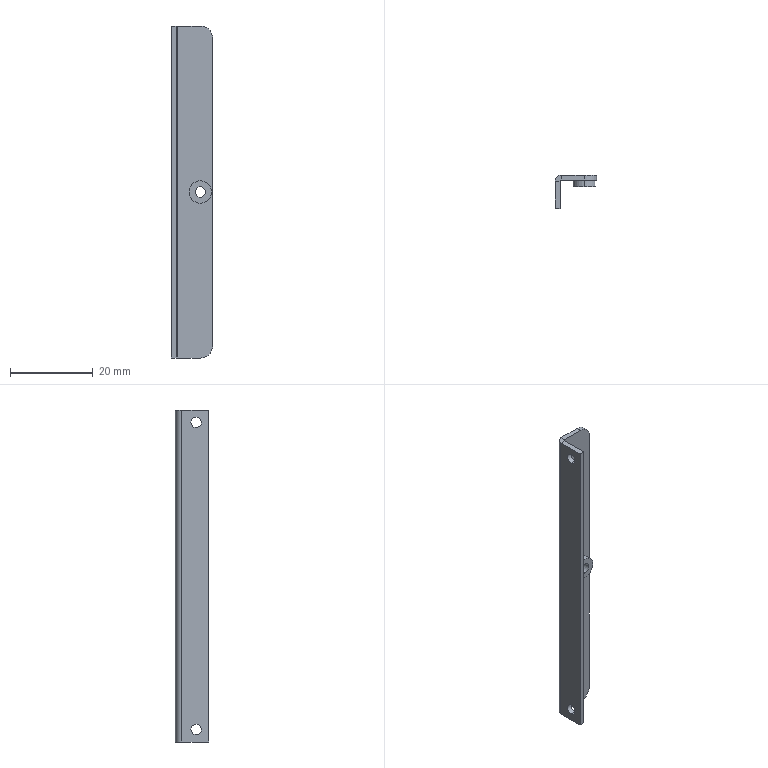Part | STEP file | 键盘盒-08^TY.NE-0002-01-014A 键盘盒-dddeger | 1 solid | 25 faces | box 10 x 8 x 80 mm | volume 1580 mm3 | plane 13 | cylinder 12 | commonest cylinder face diameters 2.5 x6 5.4 x2 6 x2 0.6 x1 3 x1